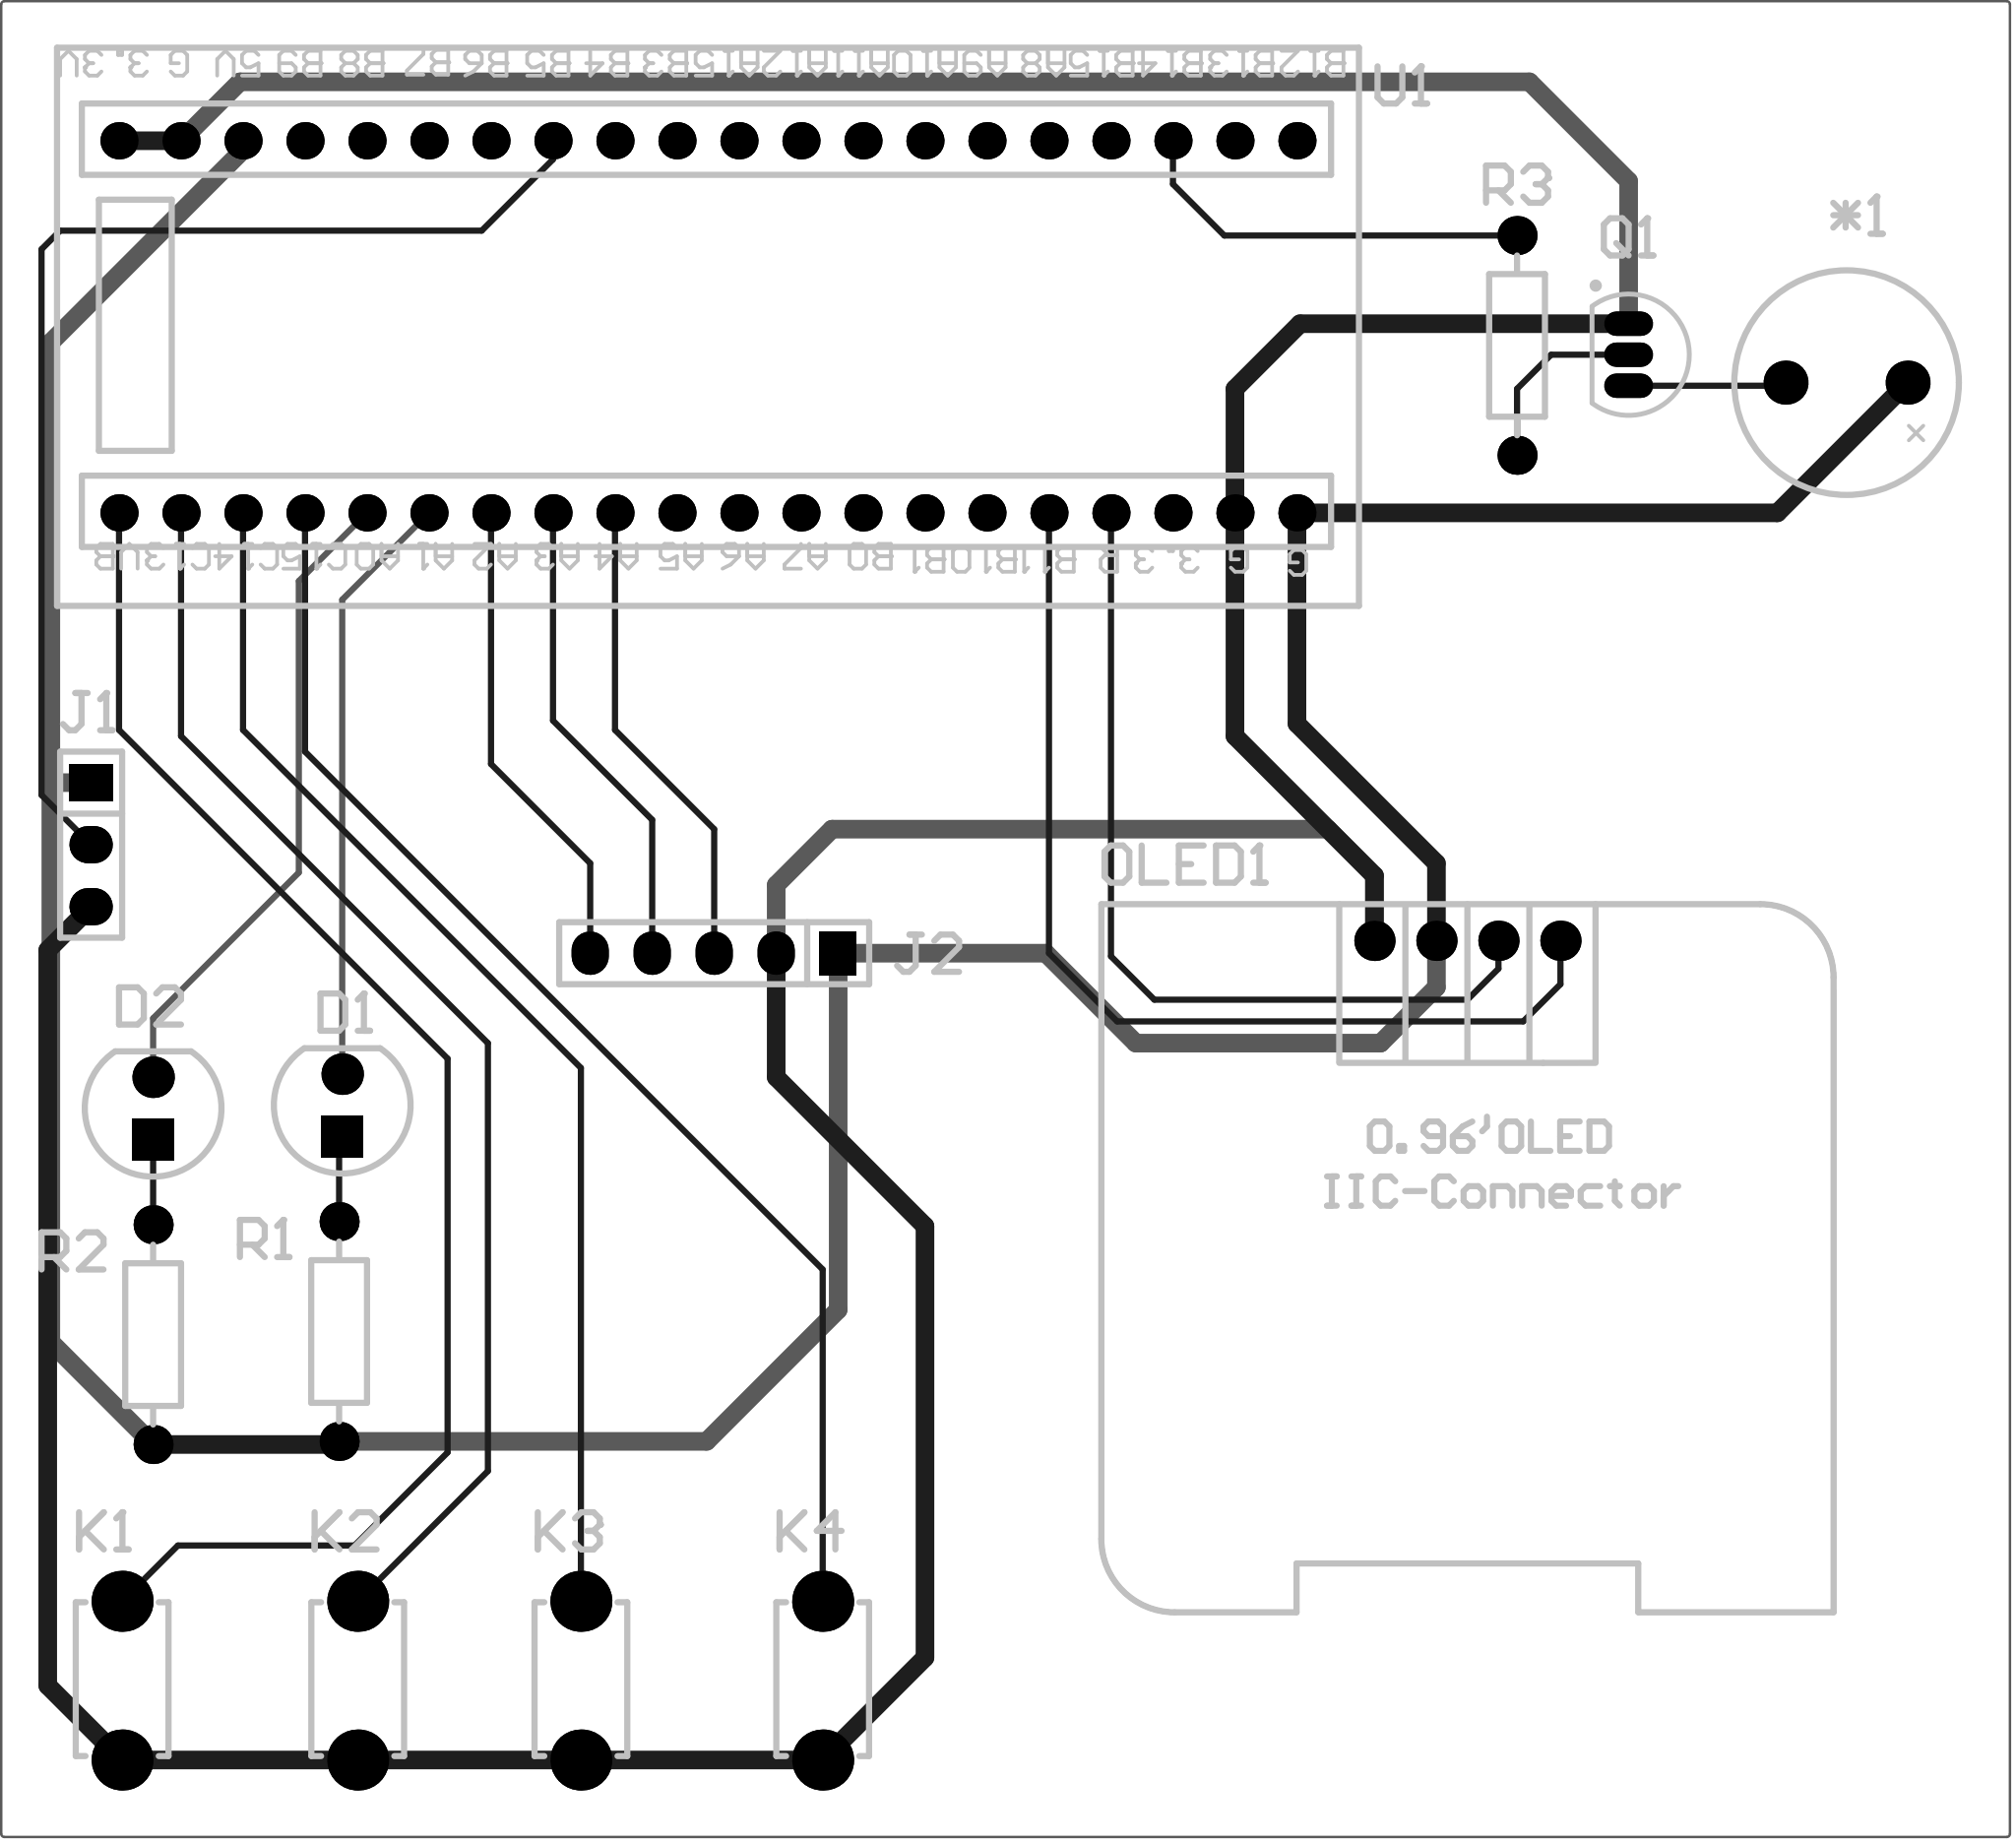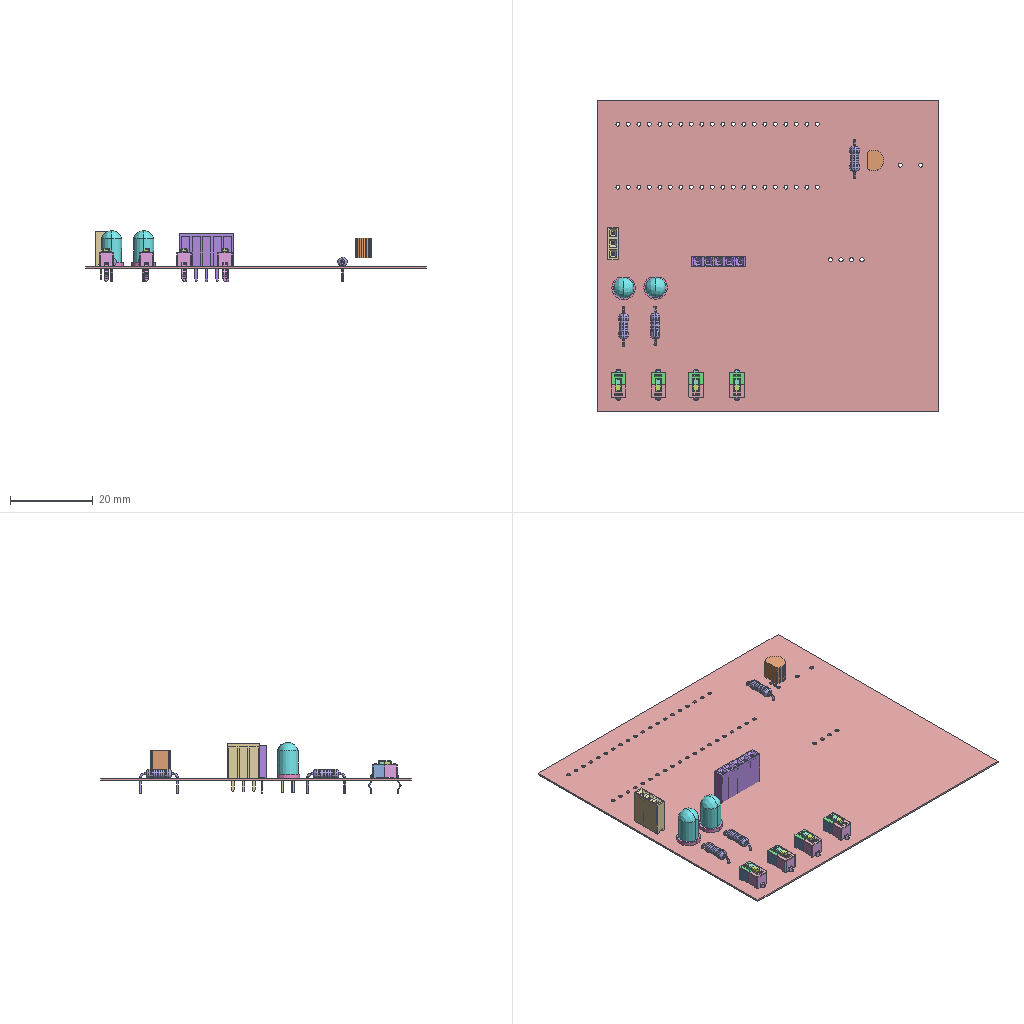Circuit board layout | Altium Designer | box 82.3 x 75.2 x 12.4 mm
Layer stack:
# Altium Designer layer stack of  (unit mm; dielectric type: 0 none, 1 core, 2 prepreg, 3 surface material)
index,name,kind,layer,copper_thickness_mm,dielectric_type,dielectric_thickness_mm,dielectric_material,dielectric_constant
0,Top Paste,other,,,,,,
1,Top Overlay,other,,,,,,
2,Top Solder,dielectric,,,3,0.0102,Solder Resist,3.5
3,Top Layer,copper,Top Layer,0.0356,,,,
4,Dielectric 1,dielectric,,,0,0.32,FR-4,4.8
5,Bottom Layer,copper,Bottom Layer,0.0356,,,,
6,Bottom Solder,dielectric,,,3,0.0102,Solder Resist,3.5
7,Bottom Overlay,other,,,,,,
8,Bottom Paste,other,,,,,,
# drill layer pairs: low layer,high layer
drill_pair,Top Layer,Bottom Layer
Part placement:
Designator,Comment,Layer,Footprint,Center-X(mm),Center-Y(mm),Rotation
*1,Buzzer,TopLayer,BUZZER,142.153,84.836,180
D1,LED,TopLayer,LED_5MM-W,80.518,55.245,90
D2,LED,TopLayer,LED_5MM-W,72.771,55.118,90
J1,DHT11,TopLayer,Fe-HDR1X3/2.54-S,70.231,65.913,0
J2,DS1302,TopLayer,Fe-HDR1X5/2.54-S,95.758,61.468,270
K1,KEY,TopLayer,DIP-3X6X4.3,71.501,31.675,90
K2,KEY,TopLayer,DIP-3X6X4.3,81.153,31.675,90
K3,KEY,TopLayer,DIP-3X6X4.3,90.297,31.675,90
K4,KEY,TopLayer,DIP-3X6X4.3,100.203,31.675,90
OLED1,0.96OLED,TopLayer,0.96OLED_4P,126.619,61.975,0
Q1,2N3904,TopLayer,TO-92A,133.223,85.979,180
R1,10K,TopLayer,RS_1/4W,80.391,45.974,90
R2,10K,TopLayer,RS_1/4W,72.771,45.847,90
R3,10K,TopLayer,RS_1/4W,128.651,86.36,270
U1,STM32F103C8T6 system board,TopLayer,STM32核心板,95.504,87.122,90
Pad and via stacks:
# Altium Designer via and pad stacks of  (unit mm). Each distinct definition once, with the count of objects using it.
# via: kind,start_layer,end_layer,hole_mm,diameter_mm,mode(0 simple;1 top-mid-bottom;2 full stack),diameter_per_layer,count,example_net
# pad: kind,layer,hole_mm,hole_type(0 round;1 square;2 slot),plating,top_size,top_shape(1 round;2 rect;3 octagon;9 rounded rect),mid_size,bottom_size,mode,footprint,size_per_layer,count,example
pad,Multi-Layer,1.2,0,plated,2.5x2.5,1,2.5x2.5,2.5x2.5,0,DIP-3X6X4.3,,8,K4.3
pad,Multi-Layer,0.9,0,plated,2x1,1,2x1,2x1,0,TO-92A,,3,Q1.1
pad,Multi-Layer,0.6,0,plated,1.6x1.6,1,1.6x1.6,1.6x1.6,0,RS 1/4W,,6,R3.1
pad,Multi-Layer,0.8128,0,plated,1.524x1.778,1,1.524x1.778,1.524x1.778,0,Fe-HDR1X5/2.54-S,,4,J2.5
pad,Multi-Layer,0.8128,0,plated,1.524x1.778,2,1.524x1.778,1.524x1.778,0,Fe-HDR1X5/2.54-S,,1,J2.1
pad,Multi-Layer,1,0,plated,1.8x1.8,1,1.8x1.8,1.8x1.8,0,BUZZER,,2,*1.2
pad,Multi-Layer,0.9,0,plated,1.7x1.7,2,1.7x1.7,1.7x1.7,0,LED 5MM-W,,2,D2.1
pad,Multi-Layer,0.9,0,plated,1.7x1.7,1,1.7x1.7,1.7x1.7,0,LED 5MM-W,,2,D2.2
pad,Multi-Layer,0.8128,0,plated,1.524x1.778,1,1.524x1.778,1.524x1.778,0,Fe-HDR1X3/2.54-S,,2,J1.3
pad,Multi-Layer,0.8128,0,plated,1.524x1.778,2,1.524x1.778,1.524x1.778,0,Fe-HDR1X3/2.54-S,,1,J1.1
pad,Multi-Layer,1,2,plated,1.65x1.65,1,1.65x1.65,1.65x1.65,0,0.96OLED_4P,,4,OLED1.1
pad,Multi-Layer,0.9144,2,plated,1.524x1.524,1,1.524x1.524,1.524x1.524,0,STM32\u00BA\u00CB\u00D0\u00C4\u00B0\u00E5,,40,U1.40
Design rules, without the lines most boards share:
# Altium Designer design rules of  (exported by Altium Designer, unit mm)
# columns: name | kind | enabled | priority | scope1 | scope2 | descriptor | typed fields (field=value)
Clearance | 0 | enabled | 1 | All | All | Clearance Constraint (Gap=10mil) (All),(All) | gap=0.254
PlaneConnect | 6 | enabled | 1 | All | All | Power Plane Connect Rule(Relief Connect )(Expansion=20mil) (Conductor Width=10mil) (Air Gap=10mil) (Entries=4) (All) | relief_conductor_width=0.254 relief_entries=4 relief_expansion=0.508
PolygonConnect | 20 | enabled | 1 | All | All | Polygon Connect Rule(Relief Connect )(Conductor Width=10mil) (Relief Angle=90 Angle) (Entries=4) (Air Gap Width=10mil) (All),(All) | connect_style(0=relief,1=direct,2=none)=0 relief_conductor_width=0.254 relief_entries=4
Width | 2 | enabled | 1 | All | All | Width Constraint (Min=10mil) (Max=30mil) (Preferred=10mil) (All) |
RoutingVias | 11 | enabled | 1 | All | All | Routing Via (MinHoleWidth=28mil) (MaxHoleWidth=28mil) (PreferredHoleWidth=28mil) (MinWidth=50mil) (MaxWidth=50mil) (PreferedWidth=50mil) (All) | via_min_hole=0.7112 via_max_hole=0.7112 via_preferred_diameter=1.27 via_preferred_hole=0.7112
PasteMaskExpansion | 14 | enabled | 1 | All | All | Paste Mask Expansion (Expansion =0mil) (All) | expansion=0
SolderMaskExpansion | 13 | enabled | 1 | All | All | Solder Mask Expansion (Expansion =4mil) (All) | expansion=0.1016
DiffPairsRouting | 51 | enabled | 1 | All | All | Differential Pairs Uncoupled Length using the Gap Constraints (Min=10mil) (Max=10mil) (Prefered=10mil)  and Width Constraints (Min=15mil) (Max=15mil) (Prefered=15mil) (All) |
HoleToHoleClearance | 52 | enabled | 1 | All | All | Hole To Hole Clearance (Gap=10mil) (All),(All) | gap=0.254
MinimumSolderMaskSliver | 53 | enabled | 1 | All | All | Minimum Solder Mask Sliver (Gap=0mil) (All),(All) |
SilkToSolderMaskClearance | 54 | enabled | 1 | IsPad | All | Silk To Solder Mask (Clearance=0mil) (IsPad),(All) |
SilkToSilkClearance | 55 | enabled | 1 | All | All | Silk to Silk (Clearance=0mil) (All),(All) |
Classes set for this board:
# Altium Designer classes of  (member kind: 0 net, 1 component, 2 from-to, 3 pad, 4 layer, 5 differential pair, 6 design channel, 7 polygon, 8 structure, 9 xSignal)
# columns: class name | member kind | superclass | members
Sheet1 | 1 | no | *1; D1; D2; J1; J2; K1; K2; K3; K4; OLED1; Q1; R1; R2; R3; U1;